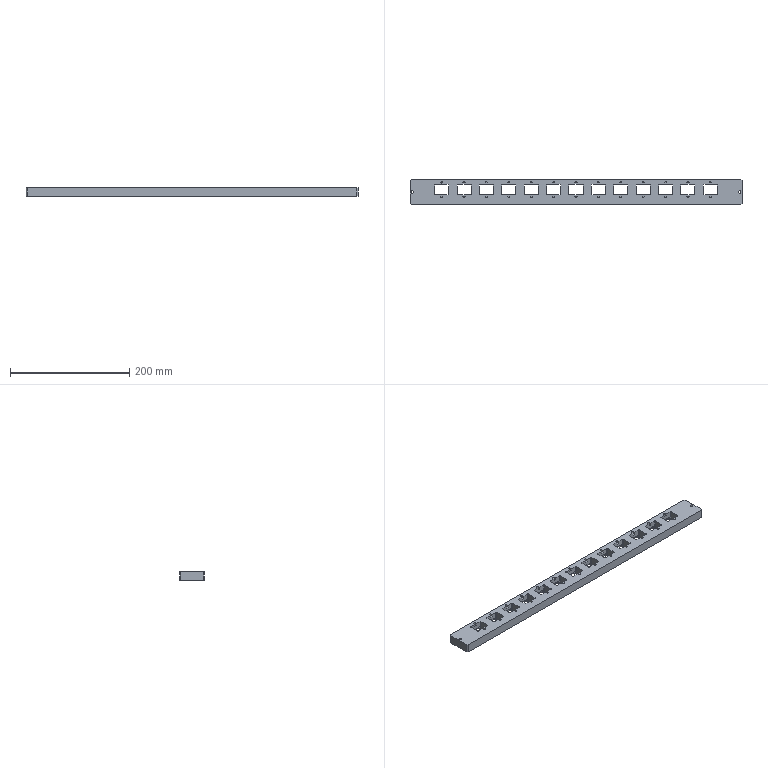NC program | NX | posted with a generic post | part box 556 x 41 x 15 mm
Lines 1305 to 2509 of 144595:
(ZLEVEL_PROFILE_COPY_1 , TOOL : D10C)
N2584 T10 M6
N2586 G54
N2588 G17 G0 G90 X218.35 Y3.984 S3500 M3
N2590 G43 Z30. H10
N2592 Z1.5
N2594 G94 G1 Y0.35 Z1.31 F1000.
N2596 X223.57 Z1.036
N2598 X224.14 Y0.282 Z1.006
N2600 X224.7 Y0.15 Z0.976
N2602 X225. Y0.04 Z0.959
N2604 X225.3 Y0.15 Z0.942
N2606 X225.86 Y0.282 Z0.912
N2608 X226.43 Y0.35 Z0.882
N2610 X231.65 Z0.608
N2612 Y7.65 Z0.226
N2614 X226.43 Z-0.048
N2616 X225.86 Y7.718 Z-0.078
N2618 X225.3 Y7.85 Z-0.108
N2620 X225. Y7.96 Z-0.125
N2622 X224.7 Y7.85 Z-0.141
N2624 X224.14 Y7.718 Z-0.172
N2626 X223.57 Y7.65 Z-0.202
N2628 X223.25 Z-0.218
N2630 X218.35 F2500.
N2632 Y0.35
N2634 X223.25
N2636 G2 X225. Y0.04 R5.1
N2638 X226.75 Y0.35 R5.1
N2640 G1 X231.65
N2642 Y7.65
N2644 X226.75
N2646 G2 X225. Y7.96 R5.1
N2648 X223.25 Y7.65 R5.1
N2650 G1 X218.35 Z-0.304
N2652 Y0.374 Z-0.431
N2654 X218.354 Y0.35
N2656 X218.661 Z-0.437
N2658 X223.25
N2660 G2 X225. Y0.04 R5.1
N2662 X226.75 Y0.35 R5.1
N2664 G1 X231.65
N2666 Y7.65
N2668 X226.75
N2670 G2 X225. Y7.96 R5.1
N2672 X223.25 Y7.65 R5.1
N2674 G1 X218.35 Z-0.522
N2676 Y0.374 Z-0.649
N2678 X218.354 Y0.35 Z-0.65
N2680 X218.661 Z-0.655
N2682 X223.25
N2684 G2 X225. Y0.04 R5.1
N2686 X226.75 Y0.35 R5.1
N2688 G1 X231.65
N2690 Y7.65
N2692 X226.75
N2694 G2 X225. Y7.96 R5.1
N2696 X223.25 Y7.65 R5.1
N2698 G1 X218.35 Z-0.741
N2700 Y0.374 Z-0.868
N2702 X218.354 Y0.35
N2704 X218.661 Z-0.874
N2706 X223.25
N2708 G2 X225. Y0.04 R5.1
N2710 X226.75 Y0.35 R5.1
N2712 G1 X231.65
N2714 Y7.65
N2716 X226.75
N2718 G2 X225. Y7.96 R5.1
N2720 X223.25 Y7.65 R5.1
N2722 G1 X218.35 Z-0.959
N2724 Y0.374 Z-1.086
N2726 X218.354 Y0.35 Z-1.087
N2728 X218.661 Z-1.092
N2730 X223.25
N2732 G2 X225. Y0.04 R5.1
N2734 X226.75 Y0.35 R5.1
N2736 G1 X231.65
N2738 Y7.65
N2740 X226.75
N2742 G2 X225. Y7.96 R5.1
N2744 X223.25 Y7.65 R5.1
N2746 G1 X218.35 Z-1.177
N2748 Y0.374 Z-1.304
N2750 X218.354 Y0.35 Z-1.305
N2752 X218.661 Z-1.31
N2754 X223.25
N2756 G2 X225. Y0.04 R5.1
N2758 X226.75 Y0.35 R5.1
N2760 G1 X231.65
N2762 Y7.65
N2764 X226.75
N2766 G2 X225. Y7.96 R5.1
N2768 X223.25 Y7.65 R5.1
N2770 G1 X218.35 Z-1.396
N2772 Y0.374 Z-1.523
N2774 X218.354 Y0.35
N2776 X218.661 Z-1.529
N2778 X223.25
N2780 G2 X225. Y0.04 R5.1
N2782 X226.75 Y0.35 R5.1
N2784 G1 X231.65
N2786 Y7.65
N2788 X226.75
N2790 G2 X225. Y7.96 R5.1
N2792 X223.25 Y7.65 R5.1
N2794 G1 X218.35 Z-1.614
N2796 Y0.374 Z-1.741
N2798 X218.354 Y0.35 Z-1.742
N2800 X218.661 Z-1.747
N2802 X223.25
N2804 G2 X225. Y0.04 R5.1
N2806 X226.75 Y0.35 R5.1
N2808 G1 X231.65
N2810 Y7.65
N2812 X226.75
N2814 G2 X225. Y7.96 R5.1
N2816 X223.25 Y7.65 R5.1
N2818 G1 X218.35 Z-1.833
N2820 Y0.374 Z-1.96
N2822 X218.354 Y0.35
N2824 X218.661 Z-1.965
N2826 X223.25
N2828 G2 X225. Y0.04 R5.1
N2830 X226.75 Y0.35 R5.1
N2832 G1 X231.65
N2834 Y7.65
N2836 X226.75
N2838 G2 X225. Y7.96 R5.1
N2840 X223.25 Y7.65 R5.1
N2842 G1 X218.35 Z-2.051
N2844 Y0.374 Z-2.178
N2846 X218.354 Y0.35
N2848 X218.661 Z-2.184
N2850 X223.25
N2852 G2 X225. Y0.04 R5.1
N2854 X226.75 Y0.35 R5.1
N2856 G1 X231.65
N2858 Y7.65
N2860 X226.75
N2862 G2 X225. Y7.96 R5.1
N2864 X223.25 Y7.65 R5.1
N2866 G1 X218.35 Z-2.269
N2868 Y0.374 Z-2.396
N2870 X218.354 Y0.35 Z-2.397
N2872 X218.661 Z-2.402
N2874 X223.25
N2876 G2 X225. Y0.04 R5.1
N2878 X226.75 Y0.35 R5.1
N2880 G1 X231.65
N2882 Y7.65
N2884 X226.75
N2886 G2 X225. Y7.96 R5.1
N2888 X223.25 Y7.65 R5.1
N2890 G1 X218.35 Z-2.488
N2892 Y0.374 Z-2.615
N2894 X218.354 Y0.35
N2896 X218.661 Z-2.621
N2898 X223.25
N2900 G2 X225. Y0.04 R5.1
N2902 X226.75 Y0.35 R5.1
N2904 G1 X231.65
N2906 Y7.65
N2908 X226.75
N2910 G2 X225. Y7.96 R5.1
N2912 X223.25 Y7.65 R5.1
N2914 G1 X218.35 Z-2.706
N2916 Y0.374 Z-2.833
N2918 X218.354 Y0.35 Z-2.834
N2920 X218.661 Z-2.839
N2922 X223.25
N2924 G2 X225. Y0.04 R5.1
N2926 X226.75 Y0.35 R5.1
N2928 G1 X231.65
N2930 Y7.65
N2932 X226.75
N2934 G2 X225. Y7.96 R5.1
N2936 X223.25 Y7.65 R5.1
N2938 G1 X218.35 Z-2.925
N2940 Y0.374 Z-3.052
N2942 X218.354 Y0.35
N2944 X218.661 Z-3.057
N2946 X223.25
N2948 G2 X225. Y0.04 R5.1
N2950 X226.75 Y0.35 R5.1
N2952 G1 X231.65
N2954 Y7.65
N2956 X226.75
N2958 G2 X225. Y7.96 R5.1
N2960 X223.25 Y7.65 R5.1
N2962 G1 X218.35 Z-3.143
N2964 Y0.374 Z-3.27
N2966 X218.354 Y0.35
N2968 X218.661 Z-3.276
N2970 X223.25
N2972 G2 X225. Y0.04 R5.1
N2974 X226.75 Y0.35 R5.1
N2976 G1 X231.65
N2978 Y7.65
N2980 X226.75
N2982 G2 X225. Y7.96 R5.1
N2984 X223.25 Y7.65 R5.1
N2986 G1 X218.35 Z-3.361
N2988 Y0.374 Z-3.488
N2990 X218.354 Y0.35 Z-3.489
N2992 X218.661 Z-3.494
N2994 X223.25
N2996 G2 X225. Y0.04 R5.1
N2998 X226.75 Y0.35 R5.1
N3000 G1 X231.65
N3002 Y7.65
N3004 X226.75
N3006 G2 X225. Y7.96 R5.1
N3008 X223.25 Y7.65 R5.1
N3010 G1 X218.35 Z-3.58
N3012 Y0.374 Z-3.707
N3014 X218.354 Y0.35
N3016 X218.661 Z-3.713
N3018 X223.25
N3020 G2 X225. Y0.04 R5.1
N3022 X226.75 Y0.35 R5.1
N3024 G1 X231.65
N3026 Y7.65
N3028 X226.75
N3030 G2 X225. Y7.96 R5.1
N3032 X223.25 Y7.65 R5.1
N3034 G1 X218.35 Z-3.798
N3036 Y0.374 Z-3.925
N3038 X218.354 Y0.35 Z-3.926
N3040 X218.661 Z-3.931
N3042 X223.25
N3044 G2 X223.781 Y0.322 R5.1
N3046 G1 X226.219
N3048 G2 X226.75 Y0.35 R5.1
N3050 G1 X231.65
N3052 Y7.65
N3054 X226.75
N3056 G2 X226.219 Y7.678 R5.1
N3058 G1 X223.781
N3060 G2 X223.25 Y7.65 R5.1
N3062 G1 X218.35 Z-4.016
N3064 Y0.374 Z-4.143
N3066 X218.354 Y0.35 Z-4.144
N3068 X218.661 Z-4.149
N3070 X231.65
N3072 Y7.65
N3074 X223.25
N3076 X218.35 Z-4.235
N3078 Y0.374 Z-4.362
N3080 X218.354 Y0.35
N3082 X218.661 Z-4.368
N3084 X231.65
N3086 Y7.65
N3088 X223.25
N3090 X218.35 Z-4.453
N3092 Y0.374 Z-4.58
N3094 X218.354 Y0.35 Z-4.581
N3096 X218.661 Z-4.586
N3098 X231.65
N3100 Y7.65
N3102 X223.25
N3104 X218.35 Z-4.672
N3106 Y0.374 Z-4.799
N3108 X218.354 Y0.35
N3110 X218.661 Z-4.804
N3112 X231.65
N3114 Y7.65
N3116 X223.25
N3118 X218.35 Z-4.89
N3120 Y0.374 Z-5.017
N3122 X218.354 Y0.35
N3124 X218.661 Z-5.023
N3126 X231.65
N3128 Y7.65
N3130 X223.25
N3132 X218.35 Z-5.108
N3134 Y0.374 Z-5.235
N3136 X218.354 Y0.35 Z-5.236
N3138 X218.661 Z-5.241
N3140 X231.65
N3142 Y7.65
N3144 X223.25
N3146 X218.35 Z-5.327
N3148 Y0.374 Z-5.454
N3150 X218.354 Y0.35
N3152 X218.661 Z-5.46
N3154 X231.65
N3156 Y7.65
N3158 X223.25
N3160 X218.35 Z-5.545
N3162 Y0.374 Z-5.672
N3164 X218.354 Y0.35 Z-5.673
N3166 X218.661 Z-5.678
N3168 X231.65
N3170 Y7.65
N3172 X223.25
N3174 X218.35 Z-5.763
N3176 Y0.374 Z-5.89
N3178 X218.354 Y0.35 Z-5.891
N3180 X218.661 Z-5.896
N3182 X231.65
N3184 Y7.65
N3186 X223.25
N3188 X218.35 Z-5.982
N3190 Y0.374 Z-6.109
N3192 X218.354 Y0.35
N3194 X218.661 Z-6.115
N3196 X231.65
N3198 Y7.65
N3200 X223.25
N3202 X218.35 Z-6.2
N3204 Y0.374 Z-6.327
N3206 X218.354 Y0.35 Z-6.328
N3208 X218.661 Z-6.333
N3210 X231.65
N3212 Y7.65
N3214 X223.25
N3216 X218.35 Z-6.419
N3218 Y0.374 Z-6.546
N3220 X218.354 Y0.35
N3222 X218.661 Z-6.551
N3224 X231.65
N3226 Y7.65
N3228 X223.25
N3230 X218.35 Z-6.637
N3232 Y0.374 Z-6.764
N3234 X218.354 Y0.35
N3236 X218.661 Z-6.77
N3238 X231.65
N3240 Y7.65
N3242 X223.25
N3244 X218.35 Z-6.855
N3246 Y0.374 Z-6.982
N3248 X218.354 Y0.35 Z-6.983
N3250 X218.661 Z-6.988
N3252 X231.65
N3254 Y7.65
N3256 X223.25
N3258 X218.35 Z-7.074
N3260 Y0.374 Z-7.201
N3262 X218.354 Y0.35
N3264 X218.661 Z-7.207
N3266 X231.65
N3268 Y7.65
N3270 X223.25
N3272 X218.35 Z-7.292
N3274 Y0.374 Z-7.419
N3276 X218.354 Y0.35 Z-7.42
N3278 X218.661 Z-7.425
N3280 X231.65
N3282 Y7.65
N3284 X223.25
N3286 X218.35 Z-7.511
N3288 Y0.374 Z-7.638
N3290 X218.354 Y0.35
N3292 X218.661 Z-7.643
N3294 X231.65
N3296 Y7.65
N3298 X223.25
N3300 X218.35 Z-7.729
N3302 Y0.374 Z-7.856
N3304 X218.354 Y0.35
N3306 X218.661 Z-7.862
N3308 X231.65
N3310 Y7.65
N3312 X223.25
N3314 X218.35 Z-7.947
N3316 Y0.374 Z-8.074
N3318 X218.354 Y0.35 Z-8.075
N3320 X218.661 Z-8.08
N3322 X231.65
N3324 Y7.65
N3326 X223.25
N3328 X218.35 Z-8.166
N3330 Y0.374 Z-8.293
N3332 X218.354 Y0.35
N3334 X218.661 Z-8.299
N3336 X231.65
N3338 Y7.65
N3340 X223.25
N3342 X218.35 Z-8.384
N3344 Y0.374 Z-8.511
N3346 X218.354 Y0.35 Z-8.512
N3348 X218.661 Z-8.517
N3350 X231.65
N3352 Y7.65
N3354 X223.25
N3356 X218.35 Z-8.602
N3358 Y0.374 Z-8.729
N3360 X218.354 Y0.35 Z-8.73
N3362 X218.661 Z-8.735
N3364 X231.65
N3366 Y7.65
N3368 X223.25
N3370 X218.35 Z-8.821
N3372 Y0.374 Z-8.948
N3374 X218.354 Y0.35
N3376 X218.661 Z-8.954
N3378 X231.65
N3380 Y7.65
N3382 X223.25
N3384 X218.35 Z-9.039
N3386 Y0.374 Z-9.166
N3388 X218.354 Y0.35 Z-9.167
N3390 X218.661 Z-9.172
N3392 X231.65
N3394 Y7.65
N3396 X223.25
N3398 X218.35 Z-9.258
N3400 Y0.374 Z-9.385
N3402 X218.354 Y0.35
N3404 X218.661 Z-9.39
N3406 X231.65
N3408 Y7.65
N3410 X223.25
N3412 X218.35 Z-9.476
N3414 Y0.374 Z-9.603
N3416 X218.354 Y0.35
N3418 X218.661 Z-9.609
N3420 X231.65
N3422 Y7.65
N3424 X223.25
N3426 X218.35 Z-9.694
N3428 Y0.374 Z-9.821
N3430 X218.354 Y0.35 Z-9.822
N3432 X218.661 Z-9.827
N3434 X231.65
N3436 Y7.65
N3438 X223.25
N3440 X218.35 Z-9.913
N3442 Y0.374 Z-10.04
N3444 X218.354 Y0.35
N3446 X218.661 Z-10.046
N3448 X231.65
N3450 Y7.65
N3452 X223.25
N3454 X218.35 Z-10.131
N3456 Y0.374 Z-10.258
N3458 X218.354 Y0.35 Z-10.259
N3460 X218.661 Z-10.264
N3462 X231.65
N3464 Y7.65
N3466 X223.25
N3468 X218.35 Z-10.35
N3470 Y0.374 Z-10.477
N3472 X218.354 Y0.35
N3474 X218.661 Z-10.482
N3476 X231.65
N3478 Y7.65
N3480 X223.25
N3482 X218.35 Z-10.568
N3484 Y0.374 Z-10.695
N3486 X218.354 Y0.35
N3488 X218.661 Z-10.701
N3490 X231.65
N3492 Y7.65
N3494 X223.25
N3496 X218.35 Z-10.786
N3498 Y0.374 Z-10.913
N3500 X218.354 Y0.35 Z-10.914
N3502 X218.661 Z-10.919
N3504 X231.65
N3506 Y7.65
N3508 X223.25
N3510 X218.35 Z-11.005
N3512 Y0.374 Z-11.132
N3514 X218.354 Y0.35
N3516 X218.661 Z-11.138
N3518 X231.65
N3520 Y7.65
N3522 X223.25
N3524 X218.35 Z-11.223
N3526 Y0.374 Z-11.35
N3528 X218.354 Y0.35 Z-11.351
N3530 X218.661 Z-11.356
N3532 X231.65
N3534 Y7.65
N3536 X223.25
N3538 X218.35 Z-11.441
N3540 Y0.374 Z-11.568
N3542 X218.354 Y0.35 Z-11.569
N3544 X218.661 Z-11.574
N3546 X231.65
N3548 Y7.65
N3550 X223.25
N3552 X218.35 Z-11.66
N3554 Y0.374 Z-11.787
N3556 X218.354 Y0.35
N3558 X218.661 Z-11.793
N3560 X231.65
N3562 Y7.65
N3564 X223.25
N3566 X218.35 Z-11.878
N3568 Y0.374 Z-12.005
N3570 X218.354 Y0.35 Z-12.006
N3572 X218.661 Z-12.011
N3574 X231.65
N3576 Y7.65
N3578 X223.25
N3580 X218.35 Z-12.097
N3582 Y0.374 Z-12.224
N3584 X218.354 Y0.35
N3586 X218.661 Z-12.229
N3588 X231.65
N3590 Y7.65
N3592 X223.25
N3594 X218.35 Z-12.315
N3596 Y0.374 Z-12.442
N3598 X218.354 Y0.35
N3600 X218.661 Z-12.448
N3602 X231.65
N3604 Y7.65
N3606 X223.25
N3608 X218.35 Z-12.533
N3610 Y0.374 Z-12.66
N3612 X218.354 Y0.35 Z-12.661
N3614 X218.661 Z-12.666
N3616 X231.65
N3618 Y7.65
N3620 X223.25
N3622 X218.35 Z-12.752
N3624 Y0.374 Z-12.879
N3626 X218.354 Y0.35
N3628 X218.661 Z-12.885
N3630 X231.65
N3632 Y7.65
N3634 X223.25
N3636 X218.35 Z-12.97
N3638 Y0.374 Z-13.097
N3640 X218.354 Y0.35 Z-13.098
N3642 X218.661 Z-13.103
N3644 X231.65
N3646 Y7.65
N3648 X223.25
N3650 X218.35 Z-13.188
N3652 Y0.374 Z-13.315
N3654 X218.354 Y0.35 Z-13.316
N3656 X218.661 Z-13.321
N3658 X231.65
N3660 Y7.65
N3662 X223.25
N3664 X218.35 Z-13.407
N3666 Y0.374 Z-13.534
N3668 X218.354 Y0.35
N3670 X218.661 Z-13.54
N3672 X231.65
N3674 Y7.65
N3676 X223.25
N3678 X218.35 Z-13.625
N3680 Y0.374 Z-13.752
N3682 X218.354 Y0.35 Z-13.753
N3684 X218.661 Z-13.758
N3686 X231.65
N3688 Y7.65
N3690 X223.25
N3692 X218.35 Z-13.844
N3694 Y0.374 Z-13.971
N3696 X218.354 Y0.35
N3698 X218.661 Z-13.976
N3700 X231.65
N3702 Y7.65
N3704 X223.25
N3706 X218.35 Z-14.062
N3708 Y0.374 Z-14.189
N3710 X218.354 Y0.35
N3712 X218.661 Z-14.195
N3714 X231.65
N3716 Y7.65
N3718 X223.25
N3720 X218.35 Z-14.28
N3722 Y0.374 Z-14.407
N3724 X218.354 Y0.35 Z-14.408
N3726 X218.661 Z-14.413
N3728 X231.65
N3730 Y7.65
N3732 X223.25
N3734 X218.35 Z-14.499
N3736 Y0.374 Z-14.626
N3738 X218.354 Y0.35
N3740 X218.661 Z-14.632
N3742 X231.65
N3744 Y7.65
N3746 X223.25
N3748 X218.35 Z-14.717
N3750 Y0.374 Z-14.844
N3752 X218.354 Y0.35 Z-14.845
N3754 X218.661 Z-14.85
N3756 X231.65
N3758 Y7.65
N3760 X218.35
N3762 Y0.35
N3764 X218.661
N3766 Z-13.35
N3768 G0 Z30.
N3770 X180.85 Y3.984
N3772 Z1.5
N3774 G1 Y0.35 Z1.31 F1000.
N3776 X186.07 Z1.036
N3778 X186.64 Y0.282 Z1.006
N3780 X187.2 Y0.15 Z0.976
N3782 X187.5 Y0.04 Z0.959
N3784 X187.8 Y0.15 Z0.942
N3786 X188.36 Y0.282 Z0.912
N3788 X188.93 Y0.35 Z0.882
N3790 X194.15 Z0.608
N3792 Y7.65 Z0.226
N3794 X188.93 Z-0.048
N3796 X188.36 Y7.718 Z-0.078
N3798 X187.8 Y7.85 Z-0.108
N3800 X187.5 Y7.96 Z-0.125
N3802 X187.2 Y7.85 Z-0.141
N3804 X186.64 Y7.718 Z-0.172
N3806 X186.07 Y7.65 Z-0.202
N3808 X185.75 Z-0.218
N3810 X180.85 F2500.
N3812 Y0.35
N3814 X185.75
N3816 G2 X187.5 Y0.04 R5.1
N3818 X189.25 Y0.35 R5.1
N3820 G1 X194.15
N3822 Y7.65
N3824 X189.25
N3826 G2 X187.5 Y7.96 R5.1
N3828 X185.75 Y7.65 R5.1
N3830 G1 X180.85 Z-0.304
N3832 Y0.374 Z-0.431
N3834 X180.854 Y0.35
N3836 X181.161 Z-0.437
N3838 X185.75
N3840 G2 X187.5 Y0.04 R5.1
N3842 X189.25 Y0.35 R5.1
N3844 G1 X194.15
N3846 Y7.65
N3848 X189.25
N3850 G2 X187.5 Y7.96 R5.1
N3852 X185.75 Y7.65 R5.1
N3854 G1 X180.85 Z-0.522
N3856 Y0.374 Z-0.649
N3858 X180.854 Y0.35 Z-0.65
N3860 X181.161 Z-0.655
N3862 X185.75
N3864 G2 X187.5 Y0.04 R5.1
N3866 X189.25 Y0.35 R5.1
N3868 G1 X194.15
N3870 Y7.65
N3872 X189.25
N3874 G2 X187.5 Y7.96 R5.1
N3876 X185.75 Y7.65 R5.1
N3878 G1 X180.85 Z-0.741
N3880 Y0.374 Z-0.868
N3882 X180.854 Y0.35
N3884 X181.161 Z-0.874
N3886 X185.75
N3888 G2 X187.5 Y0.04 R5.1
N3890 X189.25 Y0.35 R5.1
N3892 G1 X194.15
N3894 Y7.65
N3896 X189.25
N3898 G2 X187.5 Y7.96 R5.1
N3900 X185.75 Y7.65 R5.1
N3902 G1 X180.85 Z-0.959
N3904 Y0.374 Z-1.086
N3906 X180.854 Y0.35 Z-1.087
N3908 X181.161 Z-1.092
N3910 X185.75
N3912 G2 X187.5 Y0.04 R5.1
N3914 X189.25 Y0.35 R5.1
N3916 G1 X194.15
N3918 Y7.65
N3920 X189.25
N3922 G2 X187.5 Y7.96 R5.1
N3924 X185.75 Y7.65 R5.1
N3926 G1 X180.85 Z-1.177
N3928 Y0.374 Z-1.304
N3930 X180.854 Y0.35 Z-1.305
N3932 X181.161 Z-1.31
N3934 X185.75
N3936 G2 X187.5 Y0.04 R5.1
N3938 X189.25 Y0.35 R5.1
N3940 G1 X194.15
N3942 Y7.65
N3944 X189.25
N3946 G2 X187.5 Y7.96 R5.1
N3948 X185.75 Y7.65 R5.1
N3950 G1 X180.85 Z-1.396
N3952 Y0.374 Z-1.523
N3954 X180.854 Y0.35
N3956 X181.161 Z-1.529
N3958 X185.75
N3960 G2 X187.5 Y0.04 R5.1
N3962 X189.25 Y0.35 R5.1
N3964 G1 X194.15
N3966 Y7.65
N3968 X189.25
N3970 G2 X187.5 Y7.96 R5.1
N3972 X185.75 Y7.65 R5.1
N3974 G1 X180.85 Z-1.614
N3976 Y0.374 Z-1.741
N3978 X180.854 Y0.35 Z-1.742
N3980 X181.161 Z-1.747
N3982 X185.75
N3984 G2 X187.5 Y0.04 R5.1
N3986 X189.25 Y0.35 R5.1
N3988 G1 X194.15
N3990 Y7.65
N3992 X189.25
N3994 G2 X187.5 Y7.96 R5.1
N3996 X185.75 Y7.65 R5.1
N3998 G1 X180.85 Z-1.833
N4000 Y0.374 Z-1.96
N4002 X180.854 Y0.35
N4004 X181.161 Z-1.965
N4006 X185.75
N4008 G2 X187.5 Y0.04 R5.1
N4010 X189.25 Y0.35 R5.1
N4012 G1 X194.15
N4014 Y7.65
N4016 X189.25
N4018 G2 X187.5 Y7.96 R5.1
N4020 X185.75 Y7.65 R5.1
N4022 G1 X180.85 Z-2.051
N4024 Y0.374 Z-2.178
N4026 X180.854 Y0.35
N4028 X181.161 Z-2.184
N4030 X185.75
N4032 G2 X187.5 Y0.04 R5.1
N4034 X189.25 Y0.35 R5.1
N4036 G1 X194.15
N4038 Y7.65
N4040 X189.25
N4042 G2 X187.5 Y7.96 R5.1
N4044 X185.75 Y7.65 R5.1
N4046 G1 X180.85 Z-2.269
N4048 Y0.374 Z-2.396
N4050 X180.854 Y0.35 Z-2.397
N4052 X181.161 Z-2.402
N4054 X185.75
N4056 G2 X187.5 Y0.04 R5.1
N4058 X189.25 Y0.35 R5.1
N4060 G1 X194.15
N4062 Y7.65
N4064 X189.25
N4066 G2 X187.5 Y7.96 R5.1
N4068 X185.75 Y7.65 R5.1
N4070 G1 X180.85 Z-2.488
N4072 Y0.374 Z-2.615
N4074 X180.854 Y0.35
N4076 X181.161 Z-2.621
N4078 X185.75
N4080 G2 X187.5 Y0.04 R5.1
N4082 X189.25 Y0.35 R5.1
N4084 G1 X194.15
N4086 Y7.65
N4088 X189.25
N4090 G2 X187.5 Y7.96 R5.1
N4092 X185.75 Y7.65 R5.1
N4094 G1 X180.85 Z-2.706
N4096 Y0.374 Z-2.833
N4098 X180.854 Y0.35 Z-2.834
N4100 X181.161 Z-2.839
N4102 X185.75
N4104 G2 X187.5 Y0.04 R5.1
N4106 X189.25 Y0.35 R5.1
N4108 G1 X194.15
N4110 Y7.65
N4112 X189.25
N4114 G2 X187.5 Y7.96 R5.1
N4116 X185.75 Y7.65 R5.1
N4118 G1 X180.85 Z-2.925
N4120 Y0.374 Z-3.052
N4122 X180.854 Y0.35
N4124 X181.161 Z-3.057
N4126 X185.75
N4128 G2 X187.5 Y0.04 R5.1
N4130 X189.25 Y0.35 R5.1
N4132 G1 X194.15
N4134 Y7.65
N4136 X189.25
N4138 G2 X187.5 Y7.96 R5.1
N4140 X185.75 Y7.65 R5.1
N4142 G1 X180.85 Z-3.143
N4144 Y0.374 Z-3.27
N4146 X180.854 Y0.35
N4148 X181.161 Z-3.276
N4150 X185.75
N4152 G2 X187.5 Y0.04 R5.1
N4154 X189.25 Y0.35 R5.1
N4156 G1 X194.15
N4158 Y7.65
N4160 X189.25
N4162 G2 X187.5 Y7.96 R5.1
N4164 X185.75 Y7.65 R5.1
N4166 G1 X180.85 Z-3.361
N4168 Y0.374 Z-3.488
N4170 X180.854 Y0.35 Z-3.489
N4172 X181.161 Z-3.494
N4174 X185.75
N4176 G2 X187.5 Y0.04 R5.1
N4178 X189.25 Y0.35 R5.1
N4180 G1 X194.15
N4182 Y7.65
N4184 X189.25
N4186 G2 X187.5 Y7.96 R5.1
N4188 X185.75 Y7.65 R5.1
N4190 G1 X180.85 Z-3.58
N4192 Y0.374 Z-3.707
N4194 X180.854 Y0.35
N4196 X181.161 Z-3.713
N4198 X185.75
N4200 G2 X187.5 Y0.04 R5.1
N4202 X189.25 Y0.35 R5.1
N4204 G1 X194.15
N4206 Y7.65
N4208 X189.25
N4210 G2 X187.5 Y7.96 R5.1
N4212 X185.75 Y7.65 R5.1
N4214 G1 X180.85 Z-3.798
N4216 Y0.374 Z-3.925
N4218 X180.854 Y0.35 Z-3.926
N4220 X181.161 Z-3.931
N4222 X185.75
N4224 G2 X186.281 Y0.322 R5.1
N4226 G1 X188.719
N4228 G2 X189.25 Y0.35 R5.1
N4230 G1 X194.15
N4232 Y7.65
N4234 X189.25
N4236 G2 X188.719 Y7.678 R5.1
N4238 G1 X186.281
N4240 G2 X185.75 Y7.65 R5.1
N4242 G1 X180.85 Z-4.016
N4244 Y0.374 Z-4.143
N4246 X180.854 Y0.35 Z-4.144
N4248 X181.161 Z-4.149
N4250 X194.15
N4252 Y7.65
N4254 X185.75
N4256 X180.85 Z-4.235
N4258 Y0.374 Z-4.362
N4260 X180.854 Y0.35
N4262 X181.161 Z-4.368
N4264 X194.15
N4266 Y7.65
N4268 X185.75
N4270 X180.85 Z-4.453
N4272 Y0.374 Z-4.58
N4274 X180.854 Y0.35 Z-4.581
N4276 X181.161 Z-4.586
N4278 X194.15
N4280 Y7.65
N4282 X185.75
N4284 X180.85 Z-4.672
N4286 Y0.374 Z-4.799
N4288 X180.854 Y0.35
N4290 X181.161 Z-4.804
N4292 X194.15
N4294 Y7.65
N4296 X185.75
N4298 X180.85 Z-4.89
N4300 Y0.374 Z-5.017
N4302 X180.854 Y0.35
N4304 X181.161 Z-5.023
N4306 X194.15
N4308 Y7.65
N4310 X185.75
N4312 X180.85 Z-5.108
N4314 Y0.374 Z-5.235
N4316 X180.854 Y0.35 Z-5.236
N4318 X181.161 Z-5.241
N4320 X194.15
N4322 Y7.65
N4324 X185.75
N4326 X180.85 Z-5.327
N4328 Y0.374 Z-5.454
N4330 X180.854 Y0.35
N4332 X181.161 Z-5.46
N4334 X194.15
N4336 Y7.65
N4338 X185.75
N4340 X180.85 Z-5.545
N4342 Y0.374 Z-5.672
N4344 X180.854 Y0.35 Z-5.673
N4346 X181.161 Z-5.678
N4348 X194.15
N4350 Y7.65
N4352 X185.75
N4354 X180.85 Z-5.763
N4356 Y0.374 Z-5.89
N4358 X180.854 Y0.35 Z-5.891
N4360 X181.161 Z-5.896
N4362 X194.15
N4364 Y7.65
N4366 X185.75
N4368 X180.85 Z-5.982
N4370 Y0.374 Z-6.109
N4372 X180.854 Y0.35
N4374 X181.161 Z-6.115
N4376 X194.15
N4378 Y7.65
N4380 X185.75
N4382 X180.85 Z-6.2
N4384 Y0.374 Z-6.327
N4386 X180.854 Y0.35 Z-6.328
N4388 X181.161 Z-6.333
N4390 X194.15
N4392 Y7.65
N4394 X185.75
N4396 X180.85 Z-6.419
N4398 Y0.374 Z-6.546
N4400 X180.854 Y0.35
N4402 X181.161 Z-6.551
N4404 X194.15
N4406 Y7.65
N4408 X185.75
N4410 X180.85 Z-6.637
N4412 Y0.374 Z-6.764
N4414 X180.854 Y0.35
N4416 X181.161 Z-6.77
N4418 X194.15
N4420 Y7.65
N4422 X185.75
N4424 X180.85 Z-6.855
N4426 Y0.374 Z-6.982
N4428 X180.854 Y0.35 Z-6.983
N4430 X181.161 Z-6.988
N4432 X194.15
N4434 Y7.65
N4436 X185.75
N4438 X180.85 Z-7.074
N4440 Y0.374 Z-7.201
N4442 X180.854 Y0.35
N4444 X181.161 Z-7.207
N4446 X194.15
N4448 Y7.65
N4450 X185.75
N4452 X180.85 Z-7.292
N4454 Y0.374 Z-7.419
N4456 X180.854 Y0.35 Z-7.42
N4458 X181.161 Z-7.425
N4460 X194.15
N4462 Y7.65
N4464 X185.75
N4466 X180.85 Z-7.511
N4468 Y0.374 Z-7.638
N4470 X180.854 Y0.35
N4472 X181.161 Z-7.643
N4474 X194.15
N4476 Y7.65
N4478 X185.75
N4480 X180.85 Z-7.729
N4482 Y0.374 Z-7.856
N4484 X180.854 Y0.35
N4486 X181.161 Z-7.862
N4488 X194.15
N4490 Y7.65
N4492 X185.75
N4494 X180.85 Z-7.947
N4496 Y0.374 Z-8.074
N4498 X180.854 Y0.35 Z-8.075
N4500 X181.161 Z-8.08
N4502 X194.15
N4504 Y7.65
N4506 X185.75
N4508 X180.85 Z-8.166
N4510 Y0.374 Z-8.293
N4512 X180.854 Y0.35
N4514 X181.161 Z-8.299
N4516 X194.15
N4518 Y7.65
N4520 X185.75
N4522 X180.85 Z-8.384
N4524 Y0.374 Z-8.511
N4526 X180.854 Y0.35 Z-8.512
N4528 X181.161 Z-8.517
N4530 X194.15
N4532 Y7.65
N4534 X185.75
N4536 X180.85 Z-8.602
N4538 Y0.374 Z-8.729
N4540 X180.854 Y0.35 Z-8.73
N4542 X181.161 Z-8.735
N4544 X194.15
N4546 Y7.65
N4548 X185.75
N4550 X180.85 Z-8.821
N4552 Y0.374 Z-8.948
N4554 X180.854 Y0.35
N4556 X181.161 Z-8.954
N4558 X194.15
N4560 Y7.65
N4562 X185.75
N4564 X180.85 Z-9.039
N4566 Y0.374 Z-9.166
N4568 X180.854 Y0.35 Z-9.167
N4570 X181.161 Z-9.172
N4572 X194.15
N4574 Y7.65
N4576 X185.75
N4578 X180.85 Z-9.258
N4580 Y0.374 Z-9.385
N4582 X180.854 Y0.35
N4584 X181.161 Z-9.39
N4586 X194.15
N4588 Y7.65
N4590 X185.75
N4592 X180.85 Z-9.476
N4594 Y0.374 Z-9.603
N4596 X180.854 Y0.35
N4598 X181.161 Z-9.609
N4600 X194.15
N4602 Y7.65
N4604 X185.75
N4606 X180.85 Z-9.694
N4608 Y0.374 Z-9.821
N4610 X180.854 Y0.35 Z-9.822
N4612 X181.161 Z-9.827
N4614 X194.15
N4616 Y7.65
N4618 X185.75
N4620 X180.85 Z-9.913
N4622 Y0.374 Z-10.04
N4624 X180.854 Y0.35
N4626 X181.161 Z-10.046
N4628 X194.15
N4630 Y7.65
N4632 X185.75
N4634 X180.85 Z-10.131
N4636 Y0.374 Z-10.258
N4638 X180.854 Y0.35 Z-10.259
N4640 X181.161 Z-10.264
N4642 X194.15
N4644 Y7.65
N4646 X185.75
N4648 X180.85 Z-10.35
N4650 Y0.374 Z-10.477
N4652 X180.854 Y0.35
N4654 X181.161 Z-10.482
N4656 X194.15
N4658 Y7.65
N4660 X185.75
N4662 X180.85 Z-10.568
N4664 Y0.374 Z-10.695
N4666 X180.854 Y0.35
N4668 X181.161 Z-10.701
N4670 X194.15
N4672 Y7.65
N4674 X185.75
N4676 X180.85 Z-10.786
N4678 Y0.374 Z-10.913
N4680 X180.854 Y0.35 Z-10.914
N4682 X181.161 Z-10.919
N4684 X194.15
N4686 Y7.65
N4688 X185.75
N4690 X180.85 Z-11.005
N4692 Y0.374 Z-11.132
N4694 X180.854 Y0.35
N4696 X181.161 Z-11.138
N4698 X194.15
N4700 Y7.65
N4702 X185.75
N4704 X180.85 Z-11.223
N4706 Y0.374 Z-11.35
N4708 X180.854 Y0.35 Z-11.351
N4710 X181.161 Z-11.356
N4712 X194.15
N4714 Y7.65
N4716 X185.75
N4718 X180.85 Z-11.441
N4720 Y0.374 Z-11.568
N4722 X180.854 Y0.35 Z-11.569
N4724 X181.161 Z-11.574
N4726 X194.15
N4728 Y7.65
N4730 X185.75
N4732 X180.85 Z-11.66
N4734 Y0.374 Z-11.787
N4736 X180.854 Y0.35
N4738 X181.161 Z-11.793
N4740 X194.15
N4742 Y7.65
N4744 X185.75
N4746 X180.85 Z-11.878
N4748 Y0.374 Z-12.005
N4750 X180.854 Y0.35 Z-12.006
N4752 X181.161 Z-12.011
N4754 X194.15
N4756 Y7.65
N4758 X185.75
N4760 X180.85 Z-12.097
N4762 Y0.374 Z-12.224
N4764 X180.854 Y0.35
N4766 X181.161 Z-12.229
N4768 X194.15
N4770 Y7.65
N4772 X185.75
N4774 X180.85 Z-12.315
N4776 Y0.374 Z-12.442
N4778 X180.854 Y0.35
N4780 X181.161 Z-12.448
N4782 X194.15
N4784 Y7.65
N4786 X185.75
N4788 X180.85 Z-12.533
N4790 Y0.374 Z-12.66
N4792 X180.854 Y0.35 Z-12.661
N4794 X181.161 Z-12.666
N4796 X194.15
N4798 Y7.65
N4800 X185.75
N4802 X180.85 Z-12.752
N4804 Y0.374 Z-12.879
N4806 X180.854 Y0.35
N4808 X181.161 Z-12.885
N4810 X194.15
N4812 Y7.65
N4814 X185.75
N4816 X180.85 Z-12.97
N4818 Y0.374 Z-13.097
N4820 X180.854 Y0.35 Z-13.098
N4822 X181.161 Z-13.103
N4824 X194.15
N4826 Y7.65
N4828 X185.75
N4830 X180.85 Z-13.188
N4832 Y0.374 Z-13.315
N4834 X180.854 Y0.35 Z-13.316
N4836 X181.161 Z-13.321
N4838 X194.15
N4840 Y7.65
N4842 X185.75
N4844 X180.85 Z-13.407
N4846 Y0.374 Z-13.534
N4848 X180.854 Y0.35
N4850 X181.161 Z-13.54
N4852 X194.15
N4854 Y7.65
N4856 X185.75
N4858 X180.85 Z-13.625
N4860 Y0.374 Z-13.752
N4862 X180.854 Y0.35 Z-13.753
N4864 X181.161 Z-13.758
N4866 X194.15
N4868 Y7.65
N4870 X185.75
N4872 X180.85 Z-13.844
N4874 Y0.374 Z-13.971
N4876 X180.854 Y0.35
N4878 X181.161 Z-13.976
N4880 X194.15
N4882 Y7.65
N4884 X185.75
N4886 X180.85 Z-14.062
N4888 Y0.374 Z-14.189
N4890 X180.854 Y0.35
N4892 X181.161 Z-14.195
N4894 X194.15
N4896 Y7.65
N4898 X185.75
N4900 X180.85 Z-14.28
N4902 Y0.374 Z-14.407
N4904 X180.854 Y0.35 Z-14.408
N4906 X181.161 Z-14.413
N4908 X194.15
N4910 Y7.65
N4912 X185.75
N4914 X180.85 Z-14.499
N4916 Y0.374 Z-14.626
N4918 X180.854 Y0.35
N4920 X181.161 Z-14.632
N4922 X194.15
N4924 Y7.65
N4926 X185.75
N4928 X180.85 Z-14.717
N4930 Y0.374 Z-14.844
N4932 X180.854 Y0.35 Z-14.845
N4934 X181.161 Z-14.85
N4936 X194.15
N4938 Y7.65
N4940 X180.85
N4942 Y0.35
N4944 X181.161
N4946 Z-13.35
N4948 G0 Z30.
N4950 X143.35 Y3.984
N4952 Z1.5
N4954 G1 Y0.35 Z1.31 F1000.
N4956 X148.57 Z1.036
N4958 X149.14 Y0.282 Z1.006
N4960 X149.7 Y0.15 Z0.976
N4962 X150. Y0.04 Z0.959
N4964 X150.3 Y0.15 Z0.942
N4966 X150.86 Y0.282 Z0.912
N4968 X151.43 Y0.35 Z0.882
N4970 X156.65 Z0.608
N4972 Y7.65 Z0.226
N4974 X151.43 Z-0.048
N4976 X150.86 Y7.718 Z-0.078
N4978 X150.3 Y7.85 Z-0.108
N4980 X150. Y7.96 Z-0.125
N4982 X149.7 Y7.85 Z-0.141
N4984 X149.14 Y7.718 Z-0.172
N4986 X148.57 Y7.65 Z-0.202